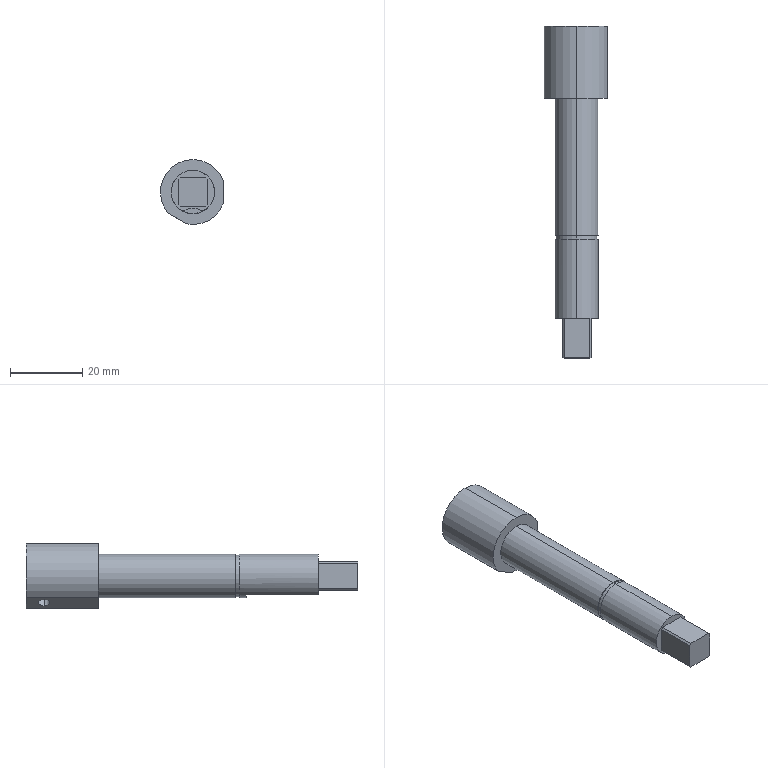Part | NX | features BREP 1 | 1 solid | 37 faces | box 17.5 x 92 x 18 mm | volume 11638 mm3 | cylinder 19 | plane 18 | commonest cylinder face diameters 3.3 x4 12 x4 1 x3 10 x3 18 x3 11.5 x2
STEP:
#1=CARTESIAN_POINT('',(2.773,20.,-5.25));
#2=VERTEX_POINT('',#1);
#3=CARTESIAN_POINT('',(2.521,20.,-5.182));
#4=VERTEX_POINT('',#3);
#5=CARTESIAN_POINT('',(2.773,20.,-4.75));
#6=DIRECTION('',(0.,1.,0.));
#7=DIRECTION('',(0.,0.,-1.));
#8=AXIS2_PLACEMENT_3D('',#5,#6,#7);
#9=CIRCLE('',#8,0.5);
#10=EDGE_CURVE('',#2,#4,#9,.T.);
#11=ORIENTED_EDGE('',*,*,#10,.F.);
#12=CARTESIAN_POINT('',(2.773,0.,-5.25));
#13=VERTEX_POINT('',#12);
#14=CARTESIAN_POINT('',(2.773,20.,-5.25));
#15=DIRECTION('',(0.,-1.,0.));
#16=VECTOR('',#15,1000.);
#17=LINE('',#14,#16);
#18=EDGE_CURVE('',#2,#13,#17,.T.);
#19=ORIENTED_EDGE('',*,*,#18,.T.);
#20=CARTESIAN_POINT('',(2.521,0.,-5.182));
#21=VERTEX_POINT('',#20);
#22=CARTESIAN_POINT('',(2.773,0.,-4.75));
#23=DIRECTION('',(0.,-1.,0.));
#24=DIRECTION('',(0.,0.,1.));
#25=AXIS2_PLACEMENT_3D('',#22,#23,#24);
#26=CIRCLE('',#25,0.5);
#27=EDGE_CURVE('',#21,#13,#26,.T.);
#28=ORIENTED_EDGE('',*,*,#27,.F.);
#29=CARTESIAN_POINT('',(2.521,20.,-5.182));
#30=DIRECTION('',(0.,-1.,0.));
#31=VECTOR('',#30,1000.);
#32=LINE('',#29,#31);
#33=EDGE_CURVE('',#4,#21,#32,.T.);
#34=ORIENTED_EDGE('',*,*,#33,.F.);
#35=EDGE_LOOP('',(#11,#19,#28,#34));
#36=FACE_BOUND('',#35,.T.);
#37=CARTESIAN_POINT('',(2.773,20.,-4.75));
#38=DIRECTION('',(0.,-1.,0.));
#39=DIRECTION('',(0.,0.,1.));
#40=AXIS2_PLACEMENT_3D('',#37,#38,#39);
#41=CYLINDRICAL_SURFACE('',#40,0.5);
#42=ADVANCED_FACE('',(#36),#41,.T.);
#43=CARTESIAN_POINT('',(-0.931,76.,-4.913));
#44=VERTEX_POINT('',#43);
#45=CARTESIAN_POINT('',(-3.789,76.,-3.263));
#46=VERTEX_POINT('',#45);
#47=CARTESIAN_POINT('',(-0.931,76.,-4.913));
#48=CARTESIAN_POINT('',(-0.931,75.561,-4.913));
#49=CARTESIAN_POINT('',(-1.313,74.711,-4.858));
#50=CARTESIAN_POINT('',(-2.532,74.169,-4.39));
#51=CARTESIAN_POINT('',(-3.552,74.711,-3.566));
#52=CARTESIAN_POINT('',(-3.789,75.561,-3.263));
#53=CARTESIAN_POINT('',(-3.789,76.,-3.263));
#54=B_SPLINE_CURVE_WITH_KNOTS('',3,(#47,#48,#49,#50,#51,#52,#53),.UNSPECIFIED.,.F.,.F.,(4,1,1,1,4),(0.,0.001298,0.002597,0.003895,0.005193),.UNSPECIFIED.);
#55=EDGE_CURVE('',#44,#46,#54,.T.);
#56=ORIENTED_EDGE('',*,*,#55,.F.);
#57=CARTESIAN_POINT('',(-2.821,76.,-8.186));
#58=VERTEX_POINT('',#57);
#59=CARTESIAN_POINT('',(-3.071,76.,-8.619));
#60=DIRECTION('',(-0.5,0.,-0.866));
#61=VECTOR('',#60,1000.);
#62=LINE('',#59,#61);
#63=EDGE_CURVE('',#58,#44,#62,.F.);
#64=ORIENTED_EDGE('',*,*,#63,.F.);
#65=CARTESIAN_POINT('',(-5.679,76.,-6.536));
#66=VERTEX_POINT('',#65);
#67=CARTESIAN_POINT('',(-4.25,76.,-7.361));
#68=DIRECTION('',(-0.5,0.,-0.866));
#69=DIRECTION('',(0.866,0.,-0.5));
#70=AXIS2_PLACEMENT_3D('',#67,#68,#69);
#71=CIRCLE('',#70,1.65);
#72=EDGE_CURVE('',#58,#66,#71,.T.);
#73=ORIENTED_EDGE('',*,*,#72,.T.);
#74=CARTESIAN_POINT('',(-5.929,76.,-6.969));
#75=DIRECTION('',(-0.5,0.,-0.866));
#76=VECTOR('',#75,1000.);
#77=LINE('',#74,#76);
#78=EDGE_CURVE('',#66,#46,#77,.F.);
#79=ORIENTED_EDGE('',*,*,#78,.T.);
#80=EDGE_LOOP('',(#56,#64,#73,#79));
#81=FACE_BOUND('',#80,.T.);
#82=CARTESIAN_POINT('',(-4.5,76.,-7.794));
#83=DIRECTION('',(-0.5,0.,-0.866));
#84=DIRECTION('',(0.866,0.,-0.5));
#85=AXIS2_PLACEMENT_3D('',#82,#83,#84);
#86=CYLINDRICAL_SURFACE('',#85,1.65);
#87=ADVANCED_FACE('',(#81),#86,.F.);
#88=CARTESIAN_POINT('',(4.72,76.,1.65));
#89=VERTEX_POINT('',#88);
#90=CARTESIAN_POINT('',(4.72,76.,-1.65));
#91=VERTEX_POINT('',#90);
#92=CARTESIAN_POINT('',(4.72,76.,1.65));
#93=CARTESIAN_POINT('',(4.72,75.561,1.65));
#94=CARTESIAN_POINT('',(4.864,74.711,1.292));
#95=CARTESIAN_POINT('',(5.068,74.169,0.002831));
#96=CARTESIAN_POINT('',(4.864,74.711,-1.293));
#97=CARTESIAN_POINT('',(4.72,75.561,-1.65));
#98=CARTESIAN_POINT('',(4.72,76.,-1.65));
#99=B_SPLINE_CURVE_WITH_KNOTS('',3,(#92,#93,#94,#95,#96,#97,#98),.UNSPECIFIED.,.F.,.F.,(4,1,1,1,4),(0.,0.001298,0.002597,0.003895,0.005193),.UNSPECIFIED.);
#100=EDGE_CURVE('',#89,#91,#99,.T.);
#101=ORIENTED_EDGE('',*,*,#100,.F.);
#102=CARTESIAN_POINT('',(8.5,76.,1.65));
#103=VERTEX_POINT('',#102);
#104=CARTESIAN_POINT('',(9.,76.,1.65));
#105=DIRECTION('',(1.,0.,0.));
#106=VECTOR('',#105,1000.);
#107=LINE('',#104,#106);
#108=EDGE_CURVE('',#103,#89,#107,.F.);
#109=ORIENTED_EDGE('',*,*,#108,.F.);
#110=CARTESIAN_POINT('',(8.5,76.,-1.65));
#111=VERTEX_POINT('',#110);
#112=CARTESIAN_POINT('',(8.5,76.,0.));
#113=DIRECTION('',(1.,0.,0.));
#114=DIRECTION('',(0.,0.,1.));
#115=AXIS2_PLACEMENT_3D('',#112,#113,#114);
#116=CIRCLE('',#115,1.65);
#117=EDGE_CURVE('',#103,#111,#116,.T.);
#118=ORIENTED_EDGE('',*,*,#117,.T.);
#119=CARTESIAN_POINT('',(9.,76.,-1.65));
#120=DIRECTION('',(1.,0.,0.));
#121=VECTOR('',#120,1000.);
#122=LINE('',#119,#121);
#123=EDGE_CURVE('',#111,#91,#122,.F.);
#124=ORIENTED_EDGE('',*,*,#123,.T.);
#125=EDGE_LOOP('',(#101,#109,#118,#124));
#126=FACE_BOUND('',#125,.T.);
#127=CARTESIAN_POINT('',(9.,76.,0.));
#128=DIRECTION('',(1.,0.,0.));
#129=DIRECTION('',(0.,0.,1.));
#130=AXIS2_PLACEMENT_3D('',#127,#128,#129);
#131=CYLINDRICAL_SURFACE('',#130,1.65);
#132=ADVANCED_FACE('',(#126),#131,.F.);
#133=CARTESIAN_POINT('',(-3.789,76.,-3.263));
#134=CARTESIAN_POINT('',(-3.789,76.439,-3.263));
#135=CARTESIAN_POINT('',(-3.551,77.289,-3.566));
#136=CARTESIAN_POINT('',(-2.536,77.831,-4.388));
#137=CARTESIAN_POINT('',(-1.312,77.289,-4.859));
#138=CARTESIAN_POINT('',(-0.931,76.439,-4.913));
#139=CARTESIAN_POINT('',(-0.931,76.,-4.913));
#140=B_SPLINE_CURVE_WITH_KNOTS('',3,(#133,#134,#135,#136,#137,#138,#139),.UNSPECIFIED.,.F.,.F.,(4,1,1,1,4),(0.,0.001298,0.002597,0.003895,0.005193),.UNSPECIFIED.);
#141=EDGE_CURVE('',#46,#44,#140,.T.);
#142=ORIENTED_EDGE('',*,*,#141,.T.);
#143=ORIENTED_EDGE('',*,*,#55,.T.);
#144=EDGE_LOOP('',(#142,#143));
#145=FACE_BOUND('',#144,.T.);
#146=CARTESIAN_POINT('',(0.,71.,-5.));
#147=VERTEX_POINT('',#146);
#148=CARTESIAN_POINT('',(0.,71.,5.));
#149=VERTEX_POINT('',#148);
#150=CARTESIAN_POINT('',(0.,71.,0.));
#151=DIRECTION('',(0.,1.,0.));
#152=DIRECTION('',(0.,0.,1.));
#153=AXIS2_PLACEMENT_3D('',#150,#151,#152);
#154=CIRCLE('',#153,5.);
#155=EDGE_CURVE('',#147,#149,#154,.T.);
#156=ORIENTED_EDGE('',*,*,#155,.F.);
#157=CARTESIAN_POINT('',(0.,81.,-5.));
#158=VERTEX_POINT('',#157);
#159=CARTESIAN_POINT('',(0.,71.,-5.));
#160=DIRECTION('',(0.,1.,0.));
#161=VECTOR('',#160,1000.);
#162=LINE('',#159,#161);
#163=EDGE_CURVE('',#147,#158,#162,.T.);
#164=ORIENTED_EDGE('',*,*,#163,.T.);
#165=CARTESIAN_POINT('',(0.,81.,5.));
#166=VERTEX_POINT('',#165);
#167=CARTESIAN_POINT('',(0.,81.,0.));
#168=DIRECTION('',(0.,1.,0.));
#169=DIRECTION('',(0.,0.,1.));
#170=AXIS2_PLACEMENT_3D('',#167,#168,#169);
#171=CIRCLE('',#170,5.);
#172=EDGE_CURVE('',#158,#166,#171,.T.);
#173=ORIENTED_EDGE('',*,*,#172,.T.);
#174=CARTESIAN_POINT('',(0.,71.,5.));
#175=DIRECTION('',(0.,1.,0.));
#176=VECTOR('',#175,1000.);
#177=LINE('',#174,#176);
#178=EDGE_CURVE('',#149,#166,#177,.T.);
#179=ORIENTED_EDGE('',*,*,#178,.F.);
#180=EDGE_LOOP('',(#156,#164,#173,#179));
#181=FACE_BOUND('',#180,.T.);
#182=CARTESIAN_POINT('',(0.,71.,0.));
#183=DIRECTION('',(0.,1.,0.));
#184=DIRECTION('',(0.,0.,-1.));
#185=AXIS2_PLACEMENT_3D('',#182,#183,#184);
#186=CYLINDRICAL_SURFACE('',#185,5.);
#187=ADVANCED_FACE('',(#145,#181),#186,.F.);
#188=CARTESIAN_POINT('',(0.,20.,-6.));
#189=VERTEX_POINT('',#188);
#190=CARTESIAN_POINT('',(3.025,20.,-5.182));
#191=VERTEX_POINT('',#190);
#192=CARTESIAN_POINT('',(0.,20.,0.));
#193=DIRECTION('',(0.,-1.,0.));
#194=DIRECTION('',(0.,0.,-1.));
#195=AXIS2_PLACEMENT_3D('',#192,#193,#194);
#196=CIRCLE('',#195,6.);
#197=EDGE_CURVE('',#189,#191,#196,.T.);
#198=ORIENTED_EDGE('',*,*,#197,.F.);
#199=CARTESIAN_POINT('',(0.,21.9,-6.));
#200=VERTEX_POINT('',#199);
#201=CARTESIAN_POINT('',(0.,128.279,-6.));
#202=DIRECTION('',(0.,1.,0.));
#203=VECTOR('',#202,1000.);
#204=LINE('',#201,#203);
#205=EDGE_CURVE('',#200,#189,#204,.F.);
#206=ORIENTED_EDGE('',*,*,#205,.F.);
#207=CARTESIAN_POINT('',(0.,21.9,6.));
#208=VERTEX_POINT('',#207);
#209=CARTESIAN_POINT('',(0.,21.9,0.));
#210=DIRECTION('',(0.,1.,0.));
#211=DIRECTION('',(0.,0.,1.));
#212=AXIS2_PLACEMENT_3D('',#209,#210,#211);
#213=CIRCLE('',#212,6.);
#214=EDGE_CURVE('',#208,#200,#213,.T.);
#215=ORIENTED_EDGE('',*,*,#214,.F.);
#216=CARTESIAN_POINT('',(0.,0.,6.));
#217=VERTEX_POINT('',#216);
#218=CARTESIAN_POINT('',(0.,128.279,6.));
#219=DIRECTION('',(0.,1.,0.));
#220=VECTOR('',#219,1000.);
#221=LINE('',#218,#220);
#222=EDGE_CURVE('',#208,#217,#221,.F.);
#223=ORIENTED_EDGE('',*,*,#222,.T.);
#224=CARTESIAN_POINT('',(3.025,0.,-5.182));
#225=VERTEX_POINT('',#224);
#226=CARTESIAN_POINT('',(0.,0.,0.));
#227=DIRECTION('',(0.,1.,0.));
#228=DIRECTION('',(0.,0.,1.));
#229=AXIS2_PLACEMENT_3D('',#226,#227,#228);
#230=CIRCLE('',#229,6.);
#231=EDGE_CURVE('',#217,#225,#230,.T.);
#232=ORIENTED_EDGE('',*,*,#231,.T.);
#233=CARTESIAN_POINT('',(3.025,128.279,-5.182));
#234=DIRECTION('',(0.,1.,0.));
#235=VECTOR('',#234,1000.);
#236=LINE('',#233,#235);
#237=EDGE_CURVE('',#225,#191,#236,.T.);
#238=ORIENTED_EDGE('',*,*,#237,.T.);
#239=EDGE_LOOP('',(#198,#206,#215,#223,#232,#238));
#240=FACE_BOUND('',#239,.T.);
#241=CARTESIAN_POINT('',(0.,128.279,0.));
#242=DIRECTION('',(0.,1.,0.));
#243=DIRECTION('',(0.,0.,-1.));
#244=AXIS2_PLACEMENT_3D('',#241,#242,#243);
#245=CYLINDRICAL_SURFACE('',#244,6.);
#246=ADVANCED_FACE('',(#240),#245,.T.);
#247=CARTESIAN_POINT('',(0.,21.9,5.75));
#248=VERTEX_POINT('',#247);
#249=CARTESIAN_POINT('',(0.,21.9,-5.75));
#250=VERTEX_POINT('',#249);
#251=CARTESIAN_POINT('',(0.,21.9,0.));
#252=DIRECTION('',(0.,1.,0.));
#253=DIRECTION('',(0.,0.,1.));
#254=AXIS2_PLACEMENT_3D('',#251,#252,#253);
#255=CIRCLE('',#254,5.75);
#256=EDGE_CURVE('',#248,#250,#255,.T.);
#257=ORIENTED_EDGE('',*,*,#256,.T.);
#258=CARTESIAN_POINT('',(0.,23.,-5.75));
#259=VERTEX_POINT('',#258);
#260=CARTESIAN_POINT('',(0.,21.9,-5.75));
#261=DIRECTION('',(0.,1.,0.));
#262=VECTOR('',#261,1000.);
#263=LINE('',#260,#262);
#264=EDGE_CURVE('',#250,#259,#263,.T.);
#265=ORIENTED_EDGE('',*,*,#264,.T.);
#266=CARTESIAN_POINT('',(0.,23.,5.75));
#267=VERTEX_POINT('',#266);
#268=CARTESIAN_POINT('',(0.,23.,0.));
#269=DIRECTION('',(0.,1.,0.));
#270=DIRECTION('',(0.,0.,1.));
#271=AXIS2_PLACEMENT_3D('',#268,#269,#270);
#272=CIRCLE('',#271,5.75);
#273=EDGE_CURVE('',#267,#259,#272,.T.);
#274=ORIENTED_EDGE('',*,*,#273,.F.);
#275=CARTESIAN_POINT('',(0.,21.9,5.75));
#276=DIRECTION('',(0.,1.,0.));
#277=VECTOR('',#276,1000.);
#278=LINE('',#275,#277);
#279=EDGE_CURVE('',#248,#267,#278,.T.);
#280=ORIENTED_EDGE('',*,*,#279,.F.);
#281=EDGE_LOOP('',(#257,#265,#274,#280));
#282=FACE_BOUND('',#281,.T.);
#283=CARTESIAN_POINT('',(0.,21.9,0.));
#284=DIRECTION('',(0.,1.,0.));
#285=DIRECTION('',(0.,0.,-1.));
#286=AXIS2_PLACEMENT_3D('',#283,#284,#285);
#287=CYLINDRICAL_SURFACE('',#286,5.75);
#288=ADVANCED_FACE('',(#282),#287,.T.);
#289=CARTESIAN_POINT('',(0.,23.,6.));
#290=VERTEX_POINT('',#289);
#291=CARTESIAN_POINT('',(0.,23.,-6.));
#292=VERTEX_POINT('',#291);
#293=CARTESIAN_POINT('',(0.,23.,0.));
#294=DIRECTION('',(0.,1.,0.));
#295=DIRECTION('',(0.,0.,1.));
#296=AXIS2_PLACEMENT_3D('',#293,#294,#295);
#297=CIRCLE('',#296,6.);
#298=EDGE_CURVE('',#290,#292,#297,.T.);
#299=ORIENTED_EDGE('',*,*,#298,.T.);
#300=CARTESIAN_POINT('',(0.,61.,-6.));
#301=VERTEX_POINT('',#300);
#302=CARTESIAN_POINT('',(0.,128.279,-6.));
#303=DIRECTION('',(0.,1.,0.));
#304=VECTOR('',#303,1000.);
#305=LINE('',#302,#304);
#306=EDGE_CURVE('',#292,#301,#305,.T.);
#307=ORIENTED_EDGE('',*,*,#306,.T.);
#308=CARTESIAN_POINT('',(0.,61.,6.));
#309=VERTEX_POINT('',#308);
#310=CARTESIAN_POINT('',(0.,61.,0.));
#311=DIRECTION('',(0.,1.,0.));
#312=DIRECTION('',(0.,0.,1.));
#313=AXIS2_PLACEMENT_3D('',#310,#311,#312);
#314=CIRCLE('',#313,6.);
#315=EDGE_CURVE('',#309,#301,#314,.T.);
#316=ORIENTED_EDGE('',*,*,#315,.F.);
#317=CARTESIAN_POINT('',(0.,128.279,6.));
#318=DIRECTION('',(0.,1.,0.));
#319=VECTOR('',#318,1000.);
#320=LINE('',#317,#319);
#321=EDGE_CURVE('',#290,#309,#320,.T.);
#322=ORIENTED_EDGE('',*,*,#321,.F.);
#323=EDGE_LOOP('',(#299,#307,#316,#322));
#324=FACE_BOUND('',#323,.T.);
#325=CARTESIAN_POINT('',(0.,128.279,0.));
#326=DIRECTION('',(0.,1.,0.));
#327=DIRECTION('',(0.,0.,-1.));
#328=AXIS2_PLACEMENT_3D('',#325,#326,#327);
#329=CYLINDRICAL_SURFACE('',#328,6.);
#330=ADVANCED_FACE('',(#324),#329,.T.);
#331=CARTESIAN_POINT('',(-6.812,61.,-5.882));
#332=VERTEX_POINT('',#331);
#333=CARTESIAN_POINT('',(0.,61.,9.));
#334=VERTEX_POINT('',#333);
#335=CARTESIAN_POINT('',(0.,61.,0.));
#336=DIRECTION('',(0.,1.,0.));
#337=DIRECTION('',(0.,0.,1.));
#338=AXIS2_PLACEMENT_3D('',#335,#336,#337);
#339=CIRCLE('',#338,9.);
#340=EDGE_CURVE('',#332,#334,#339,.T.);
#341=ORIENTED_EDGE('',*,*,#340,.T.);
#342=CARTESIAN_POINT('',(0.,81.,9.));
#343=VERTEX_POINT('',#342);
#344=CARTESIAN_POINT('',(0.,128.279,9.));
#345=DIRECTION('',(0.,1.,0.));
#346=VECTOR('',#345,1000.);
#347=LINE('',#344,#346);
#348=EDGE_CURVE('',#334,#343,#347,.T.);
#349=ORIENTED_EDGE('',*,*,#348,.T.);
#350=CARTESIAN_POINT('',(-6.812,81.,-5.882));
#351=VERTEX_POINT('',#350);
#352=CARTESIAN_POINT('',(0.,81.,0.));
#353=DIRECTION('',(0.,1.,0.));
#354=DIRECTION('',(0.,0.,1.));
#355=AXIS2_PLACEMENT_3D('',#352,#353,#354);
#356=CIRCLE('',#355,9.);
#357=EDGE_CURVE('',#351,#343,#356,.T.);
#358=ORIENTED_EDGE('',*,*,#357,.F.);
#359=CARTESIAN_POINT('',(-6.812,0.,-5.882));
#360=DIRECTION('',(0.,1.,0.));
#361=VECTOR('',#360,1000.);
#362=LINE('',#359,#361);
#363=EDGE_CURVE('',#332,#351,#362,.T.);
#364=ORIENTED_EDGE('',*,*,#363,.F.);
#365=EDGE_LOOP('',(#341,#349,#358,#364));
#366=FACE_BOUND('',#365,.T.);
#367=CARTESIAN_POINT('',(0.,128.279,0.));
#368=DIRECTION('',(0.,1.,0.));
#369=DIRECTION('',(0.,0.,-1.));
#370=AXIS2_PLACEMENT_3D('',#367,#368,#369);
#371=CYLINDRICAL_SURFACE('',#370,9.);
#372=ADVANCED_FACE('',(#366),#371,.T.);
#373=CARTESIAN_POINT('',(-3.025,0.,-5.182));
#374=VERTEX_POINT('',#373);
#375=CARTESIAN_POINT('',(0.,0.,0.));
#376=DIRECTION('',(0.,1.,0.));
#377=DIRECTION('',(0.,0.,1.));
#378=AXIS2_PLACEMENT_3D('',#375,#376,#377);
#379=CIRCLE('',#378,6.);
#380=EDGE_CURVE('',#374,#217,#379,.T.);
#381=ORIENTED_EDGE('',*,*,#380,.F.);
#382=CARTESIAN_POINT('',(-2.521,0.,-5.182));
#383=VERTEX_POINT('',#382);
#384=CARTESIAN_POINT('',(-2.773,0.,-4.75));
#385=DIRECTION('',(0.,-1.,0.));
#386=DIRECTION('',(0.,0.,1.));
#387=AXIS2_PLACEMENT_3D('',#384,#385,#386);
#388=CIRCLE('',#387,0.5);
#389=EDGE_CURVE('',#374,#383,#388,.T.);
#390=ORIENTED_EDGE('',*,*,#389,.T.);
#391=CARTESIAN_POINT('',(0.,0.,-9.5));
#392=DIRECTION('',(0.,-1.,0.));
#393=DIRECTION('',(0.,0.,-1.));
#394=AXIS2_PLACEMENT_3D('',#391,#392,#393);
#395=CIRCLE('',#394,5.);
#396=EDGE_CURVE('',#21,#383,#395,.T.);
#397=ORIENTED_EDGE('',*,*,#396,.F.);
#398=ORIENTED_EDGE('',*,*,#27,.T.);
#399=CARTESIAN_POINT('',(2.773,0.,-4.75));
#400=DIRECTION('',(0.,-1.,0.));
#401=DIRECTION('',(0.,0.,1.));
#402=AXIS2_PLACEMENT_3D('',#399,#400,#401);
#403=CIRCLE('',#402,0.5);
#404=EDGE_CURVE('',#13,#225,#403,.T.);
#405=ORIENTED_EDGE('',*,*,#404,.T.);
#406=ORIENTED_EDGE('',*,*,#231,.F.);
#407=EDGE_LOOP('',(#381,#390,#397,#398,#405,#406));
#408=FACE_BOUND('',#407,.T.);
#409=CARTESIAN_POINT('',(4.,0.,-3.5));
#410=VERTEX_POINT('',#409);
#411=CARTESIAN_POINT('',(4.,0.,3.5));
#412=VERTEX_POINT('',#411);
#413=CARTESIAN_POINT('',(4.,0.,4.));
#414=DIRECTION('',(0.,0.,1.));
#415=VECTOR('',#414,1000.);
#416=LINE('',#413,#415);
#417=EDGE_CURVE('',#410,#412,#416,.T.);
#418=ORIENTED_EDGE('',*,*,#417,.F.);
#419=CARTESIAN_POINT('',(3.5,0.,-4.));
#420=VERTEX_POINT('',#419);
#421=CARTESIAN_POINT('',(6.75,0.,-0.75));
#422=DIRECTION('',(-0.7071,0.,-0.7071));
#423=VECTOR('',#422,1000.);
#424=LINE('',#421,#423);
#425=EDGE_CURVE('',#410,#420,#424,.T.);
#426=ORIENTED_EDGE('',*,*,#425,.T.);
#427=CARTESIAN_POINT('',(-3.5,0.,-4.));
#428=VERTEX_POINT('',#427);
#429=CARTESIAN_POINT('',(-4.,0.,-4.));
#430=DIRECTION('',(1.,0.,0.));
#431=VECTOR('',#430,1000.);
#432=LINE('',#429,#431);
#433=EDGE_CURVE('',#428,#420,#432,.T.);
#434=ORIENTED_EDGE('',*,*,#433,.F.);
#435=CARTESIAN_POINT('',(-4.,0.,-3.5));
#436=VERTEX_POINT('',#435);
#437=CARTESIAN_POINT('',(-0.75,0.,-6.75));
#438=DIRECTION('',(-0.7071,0.,0.7071));
#439=VECTOR('',#438,1000.);
#440=LINE('',#437,#439);
#441=EDGE_CURVE('',#428,#436,#440,.T.);
#442=ORIENTED_EDGE('',*,*,#441,.T.);
#443=CARTESIAN_POINT('',(-4.,0.,3.5));
#444=VERTEX_POINT('',#443);
#445=CARTESIAN_POINT('',(-4.,0.,4.));
#446=DIRECTION('',(0.,0.,-1.));
#447=VECTOR('',#446,1000.);
#448=LINE('',#445,#447);
#449=EDGE_CURVE('',#444,#436,#448,.T.);
#450=ORIENTED_EDGE('',*,*,#449,.F.);
#451=CARTESIAN_POINT('',(-3.5,0.,4.));
#452=VERTEX_POINT('',#451);
#453=CARTESIAN_POINT('',(-0.75,0.,6.75));
#454=DIRECTION('',(0.7071,0.,0.7071));
#455=VECTOR('',#454,1000.);
#456=LINE('',#453,#455);
#457=EDGE_CURVE('',#444,#452,#456,.T.);
#458=ORIENTED_EDGE('',*,*,#457,.T.);
#459=CARTESIAN_POINT('',(3.5,0.,4.));
#460=VERTEX_POINT('',#459);
#461=CARTESIAN_POINT('',(-4.,0.,4.));
#462=DIRECTION('',(-1.,0.,0.));
#463=VECTOR('',#462,1000.);
#464=LINE('',#461,#463);
#465=EDGE_CURVE('',#460,#452,#464,.T.);
#466=ORIENTED_EDGE('',*,*,#465,.F.);
#467=CARTESIAN_POINT('',(6.75,0.,0.75));
#468=DIRECTION('',(0.7071,0.,-0.7071));
#469=VECTOR('',#468,1000.);
#470=LINE('',#467,#469);
#471=EDGE_CURVE('',#460,#412,#470,.T.);
#472=ORIENTED_EDGE('',*,*,#471,.T.);
#473=EDGE_LOOP('',(#418,#426,#434,#442,#450,#458,#466,#472));
#474=FACE_BOUND('',#473,.T.);
#475=CARTESIAN_POINT('',(6.,0.,0.));
#476=DIRECTION('',(0.,1.,0.));
#477=DIRECTION('',(0.,0.,-1.));
#478=AXIS2_PLACEMENT_3D('',#475,#476,#477);
#479=PLANE('',#478);
#480=ADVANCED_FACE('',(#408,#474),#479,.F.);
#481=CARTESIAN_POINT('',(8.5,61.,-2.958));
#482=VERTEX_POINT('',#481);
#483=CARTESIAN_POINT('',(-1.688,61.,-8.84));
#484=VERTEX_POINT('',#483);
#485=CARTESIAN_POINT('',(0.,61.,0.));
#486=DIRECTION('',(0.,1.,0.));
#487=DIRECTION('',(0.,0.,1.));
#488=AXIS2_PLACEMENT_3D('',#485,#486,#487);
#489=CIRCLE('',#488,9.);
#490=EDGE_CURVE('',#482,#484,#489,.T.);
#491=ORIENTED_EDGE('',*,*,#490,.T.);
#492=CARTESIAN_POINT('',(-1.688,81.,-8.84));
#493=VERTEX_POINT('',#492);
#494=CARTESIAN_POINT('',(-1.688,0.,-8.84));
#495=DIRECTION('',(0.,1.,0.));
#496=VECTOR('',#495,1000.);
#497=LINE('',#494,#496);
#498=EDGE_CURVE('',#484,#493,#497,.T.);
#499=ORIENTED_EDGE('',*,*,#498,.T.);
#500=CARTESIAN_POINT('',(8.5,81.,-2.958));
#501=VERTEX_POINT('',#500);
#502=CARTESIAN_POINT('',(0.,81.,0.));
#503=DIRECTION('',(0.,1.,0.));
#504=DIRECTION('',(0.,0.,1.));
#505=AXIS2_PLACEMENT_3D('',#502,#503,#504);
#506=CIRCLE('',#505,9.);
#507=EDGE_CURVE('',#501,#493,#506,.T.);
#508=ORIENTED_EDGE('',*,*,#507,.F.);
#509=CARTESIAN_POINT('',(8.5,0.,-2.958));
#510=DIRECTION('',(0.,1.,0.));
#511=VECTOR('',#510,1000.);
#512=LINE('',#509,#511);
#513=EDGE_CURVE('',#482,#501,#512,.T.);
#514=ORIENTED_EDGE('',*,*,#513,.F.);
#515=EDGE_LOOP('',(#491,#499,#508,#514));
#516=FACE_BOUND('',#515,.T.);
#517=CARTESIAN_POINT('',(0.,128.279,0.));
#518=DIRECTION('',(0.,1.,0.));
#519=DIRECTION('',(0.,0.,-1.));
#520=AXIS2_PLACEMENT_3D('',#517,#518,#519);
#521=CYLINDRICAL_SURFACE('',#520,9.);
#522=ADVANCED_FACE('',(#516),#521,.T.);
#523=CARTESIAN_POINT('',(0.,81.,0.));
#524=DIRECTION('',(0.,1.,0.));
#525=DIRECTION('',(0.,0.,1.));
#526=AXIS2_PLACEMENT_3D('',#523,#524,#525);
#527=CIRCLE('',#526,5.);
#528=EDGE_CURVE('',#166,#158,#527,.T.);
#529=ORIENTED_EDGE('',*,*,#528,.F.);
#530=ORIENTED_EDGE('',*,*,#172,.F.);
#531=EDGE_LOOP('',(#529,#530));
#532=FACE_BOUND('',#531,.T.);
#533=ORIENTED_EDGE('',*,*,#507,.T.);
#534=CARTESIAN_POINT('',(-6.812,81.,-5.882));
#535=DIRECTION('',(0.866,0.,-0.5));
#536=VECTOR('',#535,1000.);
#537=LINE('',#534,#536);
#538=EDGE_CURVE('',#351,#493,#537,.T.);
#539=ORIENTED_EDGE('',*,*,#538,.F.);
#540=ORIENTED_EDGE('',*,*,#357,.T.);
#541=CARTESIAN_POINT('',(8.5,81.,2.958));
#542=VERTEX_POINT('',#541);
#543=CARTESIAN_POINT('',(0.,81.,0.));
#544=DIRECTION('',(0.,1.,0.));
#545=DIRECTION('',(0.,0.,1.));
#546=AXIS2_PLACEMENT_3D('',#543,#544,#545);
#547=CIRCLE('',#546,9.);
#548=EDGE_CURVE('',#343,#542,#547,.T.);
#549=ORIENTED_EDGE('',*,*,#548,.T.);
#550=CARTESIAN_POINT('',(8.5,81.,-2.958));
#551=DIRECTION('',(0.,0.,1.));
#552=VECTOR('',#551,1000.);
#553=LINE('',#550,#552);
#554=EDGE_CURVE('',#501,#542,#553,.T.);
#555=ORIENTED_EDGE('',*,*,#554,.F.);
#556=EDGE_LOOP('',(#533,#539,#540,#549,#555));
#557=FACE_BOUND('',#556,.T.);
#558=CARTESIAN_POINT('',(0.,81.,0.));
#559=DIRECTION('',(0.,-1.,0.));
#560=DIRECTION('',(0.,0.,1.));
#561=AXIS2_PLACEMENT_3D('',#558,#559,#560);
#562=PLANE('',#561);
#563=ADVANCED_FACE('',(#532,#557),#562,.F.);
#564=ORIENTED_EDGE('',*,*,#348,.F.);
#565=CARTESIAN_POINT('',(8.5,61.,2.958));
#566=VERTEX_POINT('',#565);
#567=CARTESIAN_POINT('',(0.,61.,0.));
#568=DIRECTION('',(0.,1.,0.));
#569=DIRECTION('',(0.,0.,1.));
#570=AXIS2_PLACEMENT_3D('',#567,#568,#569);
#571=CIRCLE('',#570,9.);
#572=EDGE_CURVE('',#334,#566,#571,.T.);
#573=ORIENTED_EDGE('',*,*,#572,.T.);
#574=CARTESIAN_POINT('',(8.5,0.,2.958));
#575=DIRECTION('',(0.,1.,0.));
#576=VECTOR('',#575,1000.);
#577=LINE('',#574,#576);
#578=EDGE_CURVE('',#566,#542,#577,.T.);
#579=ORIENTED_EDGE('',*,*,#578,.T.);
#580=ORIENTED_EDGE('',*,*,#548,.F.);
#581=EDGE_LOOP('',(#564,#573,#579,#580));
#582=FACE_BOUND('',#581,.T.);
#583=CARTESIAN_POINT('',(0.,128.279,0.));
#584=DIRECTION('',(0.,1.,0.));
#585=DIRECTION('',(0.,0.,-1.));
#586=AXIS2_PLACEMENT_3D('',#583,#584,#585);
#587=CYLINDRICAL_SURFACE('',#586,9.);
#588=ADVANCED_FACE('',(#582),#587,.T.);
#589=ORIENTED_EDGE('',*,*,#340,.F.);
#590=CARTESIAN_POINT('',(2.5,61.,-11.258));
#591=DIRECTION('',(0.866,0.,-0.5));
#592=VECTOR('',#591,1000.);
#593=LINE('',#590,#592);
#594=EDGE_CURVE('',#332,#484,#593,.T.);
#595=ORIENTED_EDGE('',*,*,#594,.T.);
#596=ORIENTED_EDGE('',*,*,#490,.F.);
#597=CARTESIAN_POINT('',(8.5,61.,0.));
#598=DIRECTION('',(0.,0.,1.));
#599=VECTOR('',#598,1000.);
#600=LINE('',#597,#599);
#601=EDGE_CURVE('',#482,#566,#600,.T.);
#602=ORIENTED_EDGE('',*,*,#601,.T.);
#603=ORIENTED_EDGE('',*,*,#572,.F.);
#604=EDGE_LOOP('',(#589,#595,#596,#602,#603));
#605=FACE_BOUND('',#604,.T.);
#606=ORIENTED_EDGE('',*,*,#315,.T.);
#607=CARTESIAN_POINT('',(0.,61.,0.));
#608=DIRECTION('',(0.,1.,0.));
#609=DIRECTION('',(0.,0.,1.));
#610=AXIS2_PLACEMENT_3D('',#607,#608,#609);
#611=CIRCLE('',#610,6.);
#612=EDGE_CURVE('',#301,#309,#611,.T.);
#613=ORIENTED_EDGE('',*,*,#612,.T.);
#614=EDGE_LOOP('',(#606,#613));
#615=FACE_BOUND('',#614,.T.);
#616=CARTESIAN_POINT('',(9.,61.,0.));
#617=DIRECTION('',(0.,1.,0.));
#618=DIRECTION('',(0.,0.,-1.));
#619=AXIS2_PLACEMENT_3D('',#616,#617,#618);
#620=PLANE('',#619);
#621=ADVANCED_FACE('',(#605,#615),#620,.F.);
#622=ORIENTED_EDGE('',*,*,#306,.F.);
#623=CARTESIAN_POINT('',(0.,23.,0.));
#624=DIRECTION('',(0.,1.,0.));
#625=DIRECTION('',(0.,0.,1.));
#626=AXIS2_PLACEMENT_3D('',#623,#624,#625);
#627=CIRCLE('',#626,6.);
#628=EDGE_CURVE('',#292,#290,#627,.T.);
#629=ORIENTED_EDGE('',*,*,#628,.T.);
#630=ORIENTED_EDGE('',*,*,#321,.T.);
#631=ORIENTED_EDGE('',*,*,#612,.F.);
#632=EDGE_LOOP('',(#622,#629,#630,#631));
#633=FACE_BOUND('',#632,.T.);
#634=CARTESIAN_POINT('',(0.,128.279,0.));
#635=DIRECTION('',(0.,1.,0.));
#636=DIRECTION('',(0.,0.,-1.));
#637=AXIS2_PLACEMENT_3D('',#634,#635,#636);
#638=CYLINDRICAL_SURFACE('',#637,6.);
#639=ADVANCED_FACE('',(#633),#638,.T.);
#640=ORIENTED_EDGE('',*,*,#256,.F.);
#641=CARTESIAN_POINT('',(0.,21.9,0.));
#642=DIRECTION('',(0.,1.,0.));
#643=DIRECTION('',(0.,0.,1.));
#644=AXIS2_PLACEMENT_3D('',#641,#642,#643);
#645=CIRCLE('',#644,5.75);
#646=EDGE_CURVE('',#250,#248,#645,.T.);
#647=ORIENTED_EDGE('',*,*,#646,.F.);
#648=EDGE_LOOP('',(#640,#647));
#649=FACE_BOUND('',#648,.T.);
#650=ORIENTED_EDGE('',*,*,#214,.T.);
#651=CARTESIAN_POINT('',(0.,21.9,0.));
#652=DIRECTION('',(0.,1.,0.));
#653=DIRECTION('',(0.,0.,1.));
#654=AXIS2_PLACEMENT_3D('',#651,#652,#653);
#655=CIRCLE('',#654,6.);
#656=EDGE_CURVE('',#200,#208,#655,.T.);
#657=ORIENTED_EDGE('',*,*,#656,.T.);
#658=EDGE_LOOP('',(#650,#657));
#659=FACE_BOUND('',#658,.T.);
#660=CARTESIAN_POINT('',(0.,21.9,0.));
#661=DIRECTION('',(0.,1.,0.));
#662=DIRECTION('',(0.,0.,-1.));
#663=AXIS2_PLACEMENT_3D('',#660,#661,#662);
#664=PLANE('',#663);
#665=ADVANCED_FACE('',(#649,#659),#664,.T.);
#666=ORIENTED_EDGE('',*,*,#273,.T.);
#667=CARTESIAN_POINT('',(0.,23.,0.));
#668=DIRECTION('',(0.,1.,0.));
#669=DIRECTION('',(0.,0.,1.));
#670=AXIS2_PLACEMENT_3D('',#667,#668,#669);
#671=CIRCLE('',#670,5.75);
#672=EDGE_CURVE('',#259,#267,#671,.T.);
#673=ORIENTED_EDGE('',*,*,#672,.T.);
#674=EDGE_LOOP('',(#666,#673));
#675=FACE_BOUND('',#674,.T.);
#676=ORIENTED_EDGE('',*,*,#298,.F.);
#677=ORIENTED_EDGE('',*,*,#628,.F.);
#678=EDGE_LOOP('',(#676,#677));
#679=FACE_BOUND('',#678,.T.);
#680=CARTESIAN_POINT('',(0.,23.,0.));
#681=DIRECTION('',(0.,1.,0.));
#682=DIRECTION('',(0.,0.,-1.));
#683=AXIS2_PLACEMENT_3D('',#680,#681,#682);
#684=PLANE('',#683);
#685=ADVANCED_FACE('',(#675,#679),#684,.F.);
#686=ORIENTED_EDGE('',*,*,#264,.F.);
#687=ORIENTED_EDGE('',*,*,#646,.T.);
#688=ORIENTED_EDGE('',*,*,#279,.T.);
#689=ORIENTED_EDGE('',*,*,#672,.F.);
#690=EDGE_LOOP('',(#686,#687,#688,#689));
#691=FACE_BOUND('',#690,.T.);
#692=CARTESIAN_POINT('',(0.,21.9,0.));
#693=DIRECTION('',(0.,1.,0.));
#694=DIRECTION('',(0.,0.,-1.));
#695=AXIS2_PLACEMENT_3D('',#692,#693,#694);
#696=CYLINDRICAL_SURFACE('',#695,5.75);
#697=ADVANCED_FACE('',(#691),#696,.T.);
#698=ORIENTED_EDGE('',*,*,#205,.T.);
#699=CARTESIAN_POINT('',(-3.025,20.,-5.182));
#700=VERTEX_POINT('',#699);
#701=CARTESIAN_POINT('',(0.,20.,0.));
#702=DIRECTION('',(0.,-1.,0.));
#703=DIRECTION('',(0.,0.,-1.));
#704=AXIS2_PLACEMENT_3D('',#701,#702,#703);
#705=CIRCLE('',#704,6.);
#706=EDGE_CURVE('',#700,#189,#705,.T.);
#707=ORIENTED_EDGE('',*,*,#706,.F.);
#708=CARTESIAN_POINT('',(-3.025,128.279,-5.182));
#709=DIRECTION('',(0.,-1.,0.));
#710=VECTOR('',#709,1000.);
#711=LINE('',#708,#710);
#712=EDGE_CURVE('',#700,#374,#711,.T.);
#713=ORIENTED_EDGE('',*,*,#712,.T.);
#714=ORIENTED_EDGE('',*,*,#380,.T.);
#715=ORIENTED_EDGE('',*,*,#222,.F.);
#716=ORIENTED_EDGE('',*,*,#656,.F.);
#717=EDGE_LOOP('',(#698,#707,#713,#714,#715,#716));
#718=FACE_BOUND('',#717,.T.);
#719=CARTESIAN_POINT('',(0.,128.279,0.));
#720=DIRECTION('',(0.,1.,0.));
#721=DIRECTION('',(0.,0.,-1.));
#722=AXIS2_PLACEMENT_3D('',#719,#720,#721);
#723=CYLINDRICAL_SURFACE('',#722,6.);
#724=ADVANCED_FACE('',(#718),#723,.T.);
#725=ORIENTED_EDGE('',*,*,#163,.F.);
#726=CARTESIAN_POINT('',(0.,71.,0.));
#727=DIRECTION('',(0.,1.,0.));
#728=DIRECTION('',(0.,0.,1.));
#729=AXIS2_PLACEMENT_3D('',#726,#727,#728);
#730=CIRCLE('',#729,5.);
#731=EDGE_CURVE('',#149,#147,#730,.T.);
#732=ORIENTED_EDGE('',*,*,#731,.F.);
#733=ORIENTED_EDGE('',*,*,#178,.T.);
#734=ORIENTED_EDGE('',*,*,#528,.T.);
#735=EDGE_LOOP('',(#725,#732,#733,#734));
#736=FACE_BOUND('',#735,.T.);
#737=CARTESIAN_POINT('',(4.72,76.,-1.65));
#738=CARTESIAN_POINT('',(4.72,76.439,-1.65));
#739=CARTESIAN_POINT('',(4.864,77.289,-1.292));
#740=CARTESIAN_POINT('',(5.068,77.831,-0.002831));
#741=CARTESIAN_POINT('',(4.864,77.289,1.293));
#742=CARTESIAN_POINT('',(4.72,76.439,1.65));
#743=CARTESIAN_POINT('',(4.72,76.,1.65));
#744=B_SPLINE_CURVE_WITH_KNOTS('',3,(#737,#738,#739,#740,#741,#742,#743),.UNSPECIFIED.,.F.,.F.,(4,1,1,1,4),(0.,0.001298,0.002597,0.003895,0.005193),.UNSPECIFIED.);
#745=EDGE_CURVE('',#91,#89,#744,.T.);
#746=ORIENTED_EDGE('',*,*,#745,.T.);
#747=ORIENTED_EDGE('',*,*,#100,.T.);
#748=EDGE_LOOP('',(#746,#747));
#749=FACE_BOUND('',#748,.T.);
#750=CARTESIAN_POINT('',(0.,71.,0.));
#751=DIRECTION('',(0.,1.,0.));
#752=DIRECTION('',(0.,0.,-1.));
#753=AXIS2_PLACEMENT_3D('',#750,#751,#752);
#754=CYLINDRICAL_SURFACE('',#753,5.);
#755=ADVANCED_FACE('',(#736,#749),#754,.F.);
#756=ORIENTED_EDGE('',*,*,#731,.T.);
#757=ORIENTED_EDGE('',*,*,#155,.T.);
#758=EDGE_LOOP('',(#756,#757));
#759=FACE_BOUND('',#758,.T.);
#760=CARTESIAN_POINT('',(0.,71.,0.));
#761=DIRECTION('',(0.,1.,0.));
#762=DIRECTION('',(0.,0.,-1.));
#763=AXIS2_PLACEMENT_3D('',#760,#761,#762);
#764=PLANE('',#763);
#765=ADVANCED_FACE('',(#759),#764,.T.);
#766=ORIENTED_EDGE('',*,*,#108,.T.);
#767=ORIENTED_EDGE('',*,*,#745,.F.);
#768=ORIENTED_EDGE('',*,*,#123,.F.);
#769=CARTESIAN_POINT('',(8.5,76.,0.));
#770=DIRECTION('',(1.,0.,0.));
#771=DIRECTION('',(0.,0.,1.));
#772=AXIS2_PLACEMENT_3D('',#769,#770,#771);
#773=CIRCLE('',#772,1.65);
#774=EDGE_CURVE('',#111,#103,#773,.T.);
#775=ORIENTED_EDGE('',*,*,#774,.T.);
#776=EDGE_LOOP('',(#766,#767,#768,#775));
#777=FACE_BOUND('',#776,.T.);
#778=CARTESIAN_POINT('',(9.,76.,0.));
#779=DIRECTION('',(1.,0.,0.));
#780=DIRECTION('',(0.,0.,1.));
#781=AXIS2_PLACEMENT_3D('',#778,#779,#780);
#782=CYLINDRICAL_SURFACE('',#781,1.65);
#783=ADVANCED_FACE('',(#777),#782,.F.);
#784=ORIENTED_EDGE('',*,*,#774,.F.);
#785=ORIENTED_EDGE('',*,*,#117,.F.);
#786=EDGE_LOOP('',(#784,#785));
#787=FACE_BOUND('',#786,.T.);
#788=ORIENTED_EDGE('',*,*,#578,.F.);
#789=ORIENTED_EDGE('',*,*,#601,.F.);
#790=ORIENTED_EDGE('',*,*,#513,.T.);
#791=ORIENTED_EDGE('',*,*,#554,.T.);
#792=EDGE_LOOP('',(#788,#789,#790,#791));
#793=FACE_BOUND('',#792,.T.);
#794=CARTESIAN_POINT('',(8.5,0.,-2.958));
#795=DIRECTION('',(-1.,0.,0.));
#796=DIRECTION('',(0.,0.,-1.));
#797=AXIS2_PLACEMENT_3D('',#794,#795,#796);
#798=PLANE('',#797);
#799=ADVANCED_FACE('',(#787,#793),#798,.F.);
#800=ORIENTED_EDGE('',*,*,#63,.T.);
#801=ORIENTED_EDGE('',*,*,#141,.F.);
#802=ORIENTED_EDGE('',*,*,#78,.F.);
#803=CARTESIAN_POINT('',(-4.25,76.,-7.361));
#804=DIRECTION('',(-0.5,0.,-0.866));
#805=DIRECTION('',(0.866,0.,-0.5));
#806=AXIS2_PLACEMENT_3D('',#803,#804,#805);
#807=CIRCLE('',#806,1.65);
#808=EDGE_CURVE('',#66,#58,#807,.T.);
#809=ORIENTED_EDGE('',*,*,#808,.T.);
#810=EDGE_LOOP('',(#800,#801,#802,#809));
#811=FACE_BOUND('',#810,.T.);
#812=CARTESIAN_POINT('',(-4.5,76.,-7.794));
#813=DIRECTION('',(-0.5,0.,-0.866));
#814=DIRECTION('',(0.866,0.,-0.5));
#815=AXIS2_PLACEMENT_3D('',#812,#813,#814);
#816=CYLINDRICAL_SURFACE('',#815,1.65);
#817=ADVANCED_FACE('',(#811),#816,.F.);
#818=ORIENTED_EDGE('',*,*,#808,.F.);
#819=ORIENTED_EDGE('',*,*,#72,.F.);
#820=EDGE_LOOP('',(#818,#819));
#821=FACE_BOUND('',#820,.T.);
#822=ORIENTED_EDGE('',*,*,#498,.F.);
#823=ORIENTED_EDGE('',*,*,#594,.F.);
#824=ORIENTED_EDGE('',*,*,#363,.T.);
#825=ORIENTED_EDGE('',*,*,#538,.T.);
#826=EDGE_LOOP('',(#822,#823,#824,#825));
#827=FACE_BOUND('',#826,.T.);
#828=CARTESIAN_POINT('',(-6.812,0.,-5.882));
#829=DIRECTION('',(0.5,0.,0.866));
#830=DIRECTION('',(-0.866,0.,0.5));
#831=AXIS2_PLACEMENT_3D('',#828,#829,#830);
#832=PLANE('',#831);
#833=ADVANCED_FACE('',(#821,#827),#832,.F.);
#834=ORIENTED_EDGE('',*,*,#417,.T.);
#835=CARTESIAN_POINT('',(4.,-11.,3.5));
#836=VERTEX_POINT('',#835);
#837=CARTESIAN_POINT('',(4.,-11.,3.5));
#838=DIRECTION('',(0.,-1.,0.));
#839=VECTOR('',#838,1000.);
#840=LINE('',#837,#839);
#841=EDGE_CURVE('',#412,#836,#840,.T.);
#842=ORIENTED_EDGE('',*,*,#841,.T.);
#843=CARTESIAN_POINT('',(4.,-11.,-3.5));
#844=VERTEX_POINT('',#843);
#845=CARTESIAN_POINT('',(4.,-11.,4.));
#846=DIRECTION('',(0.,0.,1.));
#847=VECTOR('',#846,1000.);
#848=LINE('',#845,#847);
#849=EDGE_CURVE('',#844,#836,#848,.T.);
#850=ORIENTED_EDGE('',*,*,#849,.F.);
#851=CARTESIAN_POINT('',(4.,-11.,-3.5));
#852=DIRECTION('',(0.,1.,0.));
#853=VECTOR('',#852,1000.);
#854=LINE('',#851,#853);
#855=EDGE_CURVE('',#844,#410,#854,.T.);
#856=ORIENTED_EDGE('',*,*,#855,.T.);
#857=EDGE_LOOP('',(#834,#842,#850,#856));
#858=FACE_BOUND('',#857,.T.);
#859=CARTESIAN_POINT('',(4.,-11.,4.));
#860=DIRECTION('',(-1.,0.,0.));
#861=DIRECTION('',(0.,0.,-1.));
#862=AXIS2_PLACEMENT_3D('',#859,#860,#861);
#863=PLANE('',#862);
#864=ADVANCED_FACE('',(#858),#863,.F.);
#865=CARTESIAN_POINT('',(3.5,-11.,4.));
#866=VERTEX_POINT('',#865);
#867=CARTESIAN_POINT('',(-3.5,-11.,4.));
#868=VERTEX_POINT('',#867);
#869=CARTESIAN_POINT('',(-4.,-11.,4.));
#870=DIRECTION('',(-1.,0.,0.));
#871=VECTOR('',#870,1000.);
#872=LINE('',#869,#871);
#873=EDGE_CURVE('',#866,#868,#872,.T.);
#874=ORIENTED_EDGE('',*,*,#873,.F.);
#875=CARTESIAN_POINT('',(3.5,-11.,4.));
#876=DIRECTION('',(0.,1.,0.));
#877=VECTOR('',#876,1000.);
#878=LINE('',#875,#877);
#879=EDGE_CURVE('',#866,#460,#878,.T.);
#880=ORIENTED_EDGE('',*,*,#879,.T.);
#881=ORIENTED_EDGE('',*,*,#465,.T.);
#882=CARTESIAN_POINT('',(-3.5,-11.,4.));
#883=DIRECTION('',(0.,-1.,0.));
#884=VECTOR('',#883,1000.);
#885=LINE('',#882,#884);
#886=EDGE_CURVE('',#452,#868,#885,.T.);
#887=ORIENTED_EDGE('',*,*,#886,.T.);
#888=EDGE_LOOP('',(#874,#880,#881,#887));
#889=FACE_BOUND('',#888,.T.);
#890=CARTESIAN_POINT('',(-4.,-11.,4.));
#891=DIRECTION('',(0.,0.,-1.));
#892=DIRECTION('',(1.,0.,0.));
#893=AXIS2_PLACEMENT_3D('',#890,#891,#892);
#894=PLANE('',#893);
#895=ADVANCED_FACE('',(#889),#894,.F.);
#896=CARTESIAN_POINT('',(-4.,-11.,3.5));
#897=VERTEX_POINT('',#896);
#898=CARTESIAN_POINT('',(-4.,-11.,-3.5));
#899=VERTEX_POINT('',#898);
#900=CARTESIAN_POINT('',(-4.,-11.,4.));
#901=DIRECTION('',(0.,0.,-1.));
#902=VECTOR('',#901,1000.);
#903=LINE('',#900,#902);
#904=EDGE_CURVE('',#897,#899,#903,.T.);
#905=ORIENTED_EDGE('',*,*,#904,.F.);
#906=CARTESIAN_POINT('',(-4.,-11.,3.5));
#907=DIRECTION('',(0.,1.,0.));
#908=VECTOR('',#907,1000.);
#909=LINE('',#906,#908);
#910=EDGE_CURVE('',#897,#444,#909,.T.);
#911=ORIENTED_EDGE('',*,*,#910,.T.);
#912=ORIENTED_EDGE('',*,*,#449,.T.);
#913=CARTESIAN_POINT('',(-4.,-11.,-3.5));
#914=DIRECTION('',(0.,-1.,0.));
#915=VECTOR('',#914,1000.);
#916=LINE('',#913,#915);
#917=EDGE_CURVE('',#436,#899,#916,.T.);
#918=ORIENTED_EDGE('',*,*,#917,.T.);
#919=EDGE_LOOP('',(#905,#911,#912,#918));
#920=FACE_BOUND('',#919,.T.);
#921=CARTESIAN_POINT('',(-4.,-11.,4.));
#922=DIRECTION('',(1.,0.,0.));
#923=DIRECTION('',(0.,0.,1.));
#924=AXIS2_PLACEMENT_3D('',#921,#922,#923);
#925=PLANE('',#924);
#926=ADVANCED_FACE('',(#920),#925,.F.);
#927=ORIENTED_EDGE('',*,*,#433,.T.);
#928=CARTESIAN_POINT('',(3.5,-11.,-4.));
#929=VERTEX_POINT('',#928);
#930=CARTESIAN_POINT('',(3.5,-11.,-4.));
#931=DIRECTION('',(0.,-1.,0.));
#932=VECTOR('',#931,1000.);
#933=LINE('',#930,#932);
#934=EDGE_CURVE('',#420,#929,#933,.T.);
#935=ORIENTED_EDGE('',*,*,#934,.T.);
#936=CARTESIAN_POINT('',(-3.5,-11.,-4.));
#937=VERTEX_POINT('',#936);
#938=CARTESIAN_POINT('',(-4.,-11.,-4.));
#939=DIRECTION('',(1.,0.,0.));
#940=VECTOR('',#939,1000.);
#941=LINE('',#938,#940);
#942=EDGE_CURVE('',#937,#929,#941,.T.);
#943=ORIENTED_EDGE('',*,*,#942,.F.);
#944=CARTESIAN_POINT('',(-3.5,-11.,-4.));
#945=DIRECTION('',(0.,1.,0.));
#946=VECTOR('',#945,1000.);
#947=LINE('',#944,#946);
#948=EDGE_CURVE('',#937,#428,#947,.T.);
#949=ORIENTED_EDGE('',*,*,#948,.T.);
#950=EDGE_LOOP('',(#927,#935,#943,#949));
#951=FACE_BOUND('',#950,.T.);
#952=CARTESIAN_POINT('',(-4.,-11.,-4.));
#953=DIRECTION('',(0.,0.,1.));
#954=DIRECTION('',(-1.,0.,0.));
#955=AXIS2_PLACEMENT_3D('',#952,#953,#954);
#956=PLANE('',#955);
#957=ADVANCED_FACE('',(#951),#956,.F.);
#958=ORIENTED_EDGE('',*,*,#849,.T.);
#959=CARTESIAN_POINT('',(3.75,-11.,3.75));
#960=DIRECTION('',(-0.7071,0.,0.7071));
#961=VECTOR('',#960,1000.);
#962=LINE('',#959,#961);
#963=EDGE_CURVE('',#836,#866,#962,.T.);
#964=ORIENTED_EDGE('',*,*,#963,.T.);
#965=ORIENTED_EDGE('',*,*,#873,.T.);
#966=CARTESIAN_POINT('',(-3.75,-11.,3.75));
#967=DIRECTION('',(-0.7071,0.,-0.7071));
#968=VECTOR('',#967,1000.);
#969=LINE('',#966,#968);
#970=EDGE_CURVE('',#868,#897,#969,.T.);
#971=ORIENTED_EDGE('',*,*,#970,.T.);
#972=ORIENTED_EDGE('',*,*,#904,.T.);
#973=CARTESIAN_POINT('',(-3.75,-11.,-3.75));
#974=DIRECTION('',(0.7071,0.,-0.7071));
#975=VECTOR('',#974,1000.);
#976=LINE('',#973,#975);
#977=EDGE_CURVE('',#899,#937,#976,.T.);
#978=ORIENTED_EDGE('',*,*,#977,.T.);
#979=ORIENTED_EDGE('',*,*,#942,.T.);
#980=CARTESIAN_POINT('',(3.75,-11.,-3.75));
#981=DIRECTION('',(0.7071,0.,0.7071));
#982=VECTOR('',#981,1000.);
#983=LINE('',#980,#982);
#984=EDGE_CURVE('',#929,#844,#983,.T.);
#985=ORIENTED_EDGE('',*,*,#984,.T.);
#986=EDGE_LOOP('',(#958,#964,#965,#971,#972,#978,#979,#985));
#987=FACE_BOUND('',#986,.T.);
#988=CARTESIAN_POINT('',(0.,-11.,0.));
#989=DIRECTION('',(0.,-1.,0.));
#990=DIRECTION('',(0.,0.,1.));
#991=AXIS2_PLACEMENT_3D('',#988,#989,#990);
#992=PLANE('',#991);
#993=ADVANCED_FACE('',(#987),#992,.T.);
#994=ORIENTED_EDGE('',*,*,#396,.T.);
#995=CARTESIAN_POINT('',(-2.521,20.,-5.182));
#996=VERTEX_POINT('',#995);
#997=CARTESIAN_POINT('',(-2.521,20.,-5.182));
#998=DIRECTION('',(0.,1.,0.));
#999=VECTOR('',#998,1000.);
#1000=LINE('',#997,#999);
#1001=EDGE_CURVE('',#383,#996,#1000,.T.);
#1002=ORIENTED_EDGE('',*,*,#1001,.T.);
#1003=CARTESIAN_POINT('',(0.,20.,-9.5));
#1004=DIRECTION('',(0.,-1.,0.));
#1005=DIRECTION('',(0.,0.,-1.));
#1006=AXIS2_PLACEMENT_3D('',#1003,#1004,#1005);
#1007=CIRCLE('',#1006,5.);
#1008=EDGE_CURVE('',#4,#996,#1007,.T.);
#1009=ORIENTED_EDGE('',*,*,#1008,.F.);
#1010=ORIENTED_EDGE('',*,*,#33,.T.);
#1011=EDGE_LOOP('',(#994,#1002,#1009,#1010));
#1012=FACE_BOUND('',#1011,.T.);
#1013=CARTESIAN_POINT('',(0.,20.,-9.5));
#1014=DIRECTION('',(0.,-1.,0.));
#1015=DIRECTION('',(0.,0.,1.));
#1016=AXIS2_PLACEMENT_3D('',#1013,#1014,#1015);
#1017=CYLINDRICAL_SURFACE('',#1016,5.);
#1018=ADVANCED_FACE('',(#1012),#1017,.F.);
#1019=ORIENTED_EDGE('',*,*,#706,.T.);
#1020=ORIENTED_EDGE('',*,*,#197,.T.);
#1021=CARTESIAN_POINT('',(2.773,20.,-4.75));
#1022=DIRECTION('',(0.,1.,0.));
#1023=DIRECTION('',(0.,0.,-1.));
#1024=AXIS2_PLACEMENT_3D('',#1021,#1022,#1023);
#1025=CIRCLE('',#1024,0.5);
#1026=EDGE_CURVE('',#191,#2,#1025,.T.);
#1027=ORIENTED_EDGE('',*,*,#1026,.T.);
#1028=ORIENTED_EDGE('',*,*,#10,.T.);
#1029=ORIENTED_EDGE('',*,*,#1008,.T.);
#1030=CARTESIAN_POINT('',(-2.773,20.,-4.75));
#1031=DIRECTION('',(0.,1.,0.));
#1032=DIRECTION('',(0.,0.,-1.));
#1033=AXIS2_PLACEMENT_3D('',#1030,#1031,#1032);
#1034=CIRCLE('',#1033,0.5);
#1035=EDGE_CURVE('',#996,#700,#1034,.T.);
#1036=ORIENTED_EDGE('',*,*,#1035,.T.);
#1037=EDGE_LOOP('',(#1019,#1020,#1027,#1028,#1029,#1036));
#1038=FACE_BOUND('',#1037,.T.);
#1039=CARTESIAN_POINT('',(0.,20.,-9.5));
#1040=DIRECTION('',(0.,-1.,0.));
#1041=DIRECTION('',(0.,0.,1.));
#1042=AXIS2_PLACEMENT_3D('',#1039,#1040,#1041);
#1043=PLANE('',#1042);
#1044=ADVANCED_FACE('',(#1038),#1043,.T.);
#1045=ORIENTED_EDGE('',*,*,#1035,.F.);
#1046=ORIENTED_EDGE('',*,*,#1001,.F.);
#1047=ORIENTED_EDGE('',*,*,#389,.F.);
#1048=ORIENTED_EDGE('',*,*,#712,.F.);
#1049=EDGE_LOOP('',(#1045,#1046,#1047,#1048));
#1050=FACE_BOUND('',#1049,.T.);
#1051=CARTESIAN_POINT('',(-2.773,20.,-4.75));
#1052=DIRECTION('',(0.,1.,0.));
#1053=DIRECTION('',(0.,0.,-1.));
#1054=AXIS2_PLACEMENT_3D('',#1051,#1052,#1053);
#1055=CYLINDRICAL_SURFACE('',#1054,0.5);
#1056=ADVANCED_FACE('',(#1050),#1055,.T.);
#1057=ORIENTED_EDGE('',*,*,#18,.F.);
#1058=ORIENTED_EDGE('',*,*,#1026,.F.);
#1059=ORIENTED_EDGE('',*,*,#237,.F.);
#1060=ORIENTED_EDGE('',*,*,#404,.F.);
#1061=EDGE_LOOP('',(#1057,#1058,#1059,#1060));
#1062=FACE_BOUND('',#1061,.T.);
#1063=CARTESIAN_POINT('',(2.773,20.,-4.75));
#1064=DIRECTION('',(0.,-1.,0.));
#1065=DIRECTION('',(0.,0.,1.));
#1066=AXIS2_PLACEMENT_3D('',#1063,#1064,#1065);
#1067=CYLINDRICAL_SURFACE('',#1066,0.5);
#1068=ADVANCED_FACE('',(#1062),#1067,.T.);
#1069=ORIENTED_EDGE('',*,*,#963,.F.);
#1070=ORIENTED_EDGE('',*,*,#841,.F.);
#1071=ORIENTED_EDGE('',*,*,#471,.F.);
#1072=ORIENTED_EDGE('',*,*,#879,.F.);
#1073=EDGE_LOOP('',(#1069,#1070,#1071,#1072));
#1074=FACE_BOUND('',#1073,.T.);
#1075=CARTESIAN_POINT('',(3.5,-11.,4.));
#1076=DIRECTION('',(-0.7071,0.,-0.7071));
#1077=DIRECTION('',(0.,-1.,0.));
#1078=AXIS2_PLACEMENT_3D('',#1075,#1076,#1077);
#1079=PLANE('',#1078);
#1080=ADVANCED_FACE('',(#1074),#1079,.F.);
#1081=ORIENTED_EDGE('',*,*,#970,.F.);
#1082=ORIENTED_EDGE('',*,*,#886,.F.);
#1083=ORIENTED_EDGE('',*,*,#457,.F.);
#1084=ORIENTED_EDGE('',*,*,#910,.F.);
#1085=EDGE_LOOP('',(#1081,#1082,#1083,#1084));
#1086=FACE_BOUND('',#1085,.T.);
#1087=CARTESIAN_POINT('',(-4.,-11.,3.5));
#1088=DIRECTION('',(0.7071,0.,-0.7071));
#1089=DIRECTION('',(0.,-1.,0.));
#1090=AXIS2_PLACEMENT_3D('',#1087,#1088,#1089);
#1091=PLANE('',#1090);
#1092=ADVANCED_FACE('',(#1086),#1091,.F.);
#1093=ORIENTED_EDGE('',*,*,#984,.F.);
#1094=ORIENTED_EDGE('',*,*,#934,.F.);
#1095=ORIENTED_EDGE('',*,*,#425,.F.);
#1096=ORIENTED_EDGE('',*,*,#855,.F.);
#1097=EDGE_LOOP('',(#1093,#1094,#1095,#1096));
#1098=FACE_BOUND('',#1097,.T.);
#1099=CARTESIAN_POINT('',(4.,-11.,-3.5));
#1100=DIRECTION('',(-0.7071,0.,0.7071));
#1101=DIRECTION('',(0.,-1.,0.));
#1102=AXIS2_PLACEMENT_3D('',#1099,#1100,#1101);
#1103=PLANE('',#1102);
#1104=ADVANCED_FACE('',(#1098),#1103,.F.);
#1105=ORIENTED_EDGE('',*,*,#977,.F.);
#1106=ORIENTED_EDGE('',*,*,#917,.F.);
#1107=ORIENTED_EDGE('',*,*,#441,.F.);
#1108=ORIENTED_EDGE('',*,*,#948,.F.);
#1109=EDGE_LOOP('',(#1105,#1106,#1107,#1108));
#1110=FACE_BOUND('',#1109,.T.);
#1111=CARTESIAN_POINT('',(-3.5,-11.,-4.));
#1112=DIRECTION('',(0.7071,0.,0.7071));
#1113=DIRECTION('',(0.,-1.,0.));
#1114=AXIS2_PLACEMENT_3D('',#1111,#1112,#1113);
#1115=PLANE('',#1114);
#1116=ADVANCED_FACE('',(#1110),#1115,.F.);
#1117=CLOSED_SHELL('',(#42,#87,#132,#187,#246,#288,#330,#372,#480,#522,#563,#588,#621,#639,#665,#685,#697,#724,#755,#765,#783,#799,#817,#833,#864,#895,#926,#957,#993,#1018,#1044,#1056,#1068,#1080,#1092,#1104,#1116));
#1118=MANIFOLD_SOLID_BREP('',#1117);
#1119=(LENGTH_UNIT()NAMED_UNIT(*)SI_UNIT(.MILLI.,.METRE.));
#1120=UNCERTAINTY_MEASURE_WITH_UNIT(LENGTH_MEASURE(0.0508),#1119,'','');
#1121=(NAMED_UNIT(*)PLANE_ANGLE_UNIT()SI_UNIT($,.RADIAN.));
#1122=(NAMED_UNIT(*)SI_UNIT($,.STERADIAN.)SOLID_ANGLE_UNIT());
#1123=(GEOMETRIC_REPRESENTATION_CONTEXT(3)GLOBAL_UNCERTAINTY_ASSIGNED_CONTEXT((#1120))GLOBAL_UNIT_ASSIGNED_CONTEXT((#1119,#1121,#1122))REPRESENTATION_CONTEXT('',''));
#1124=ADVANCED_BREP_SHAPE_REPRESENTATION('',(#1118),#1123);